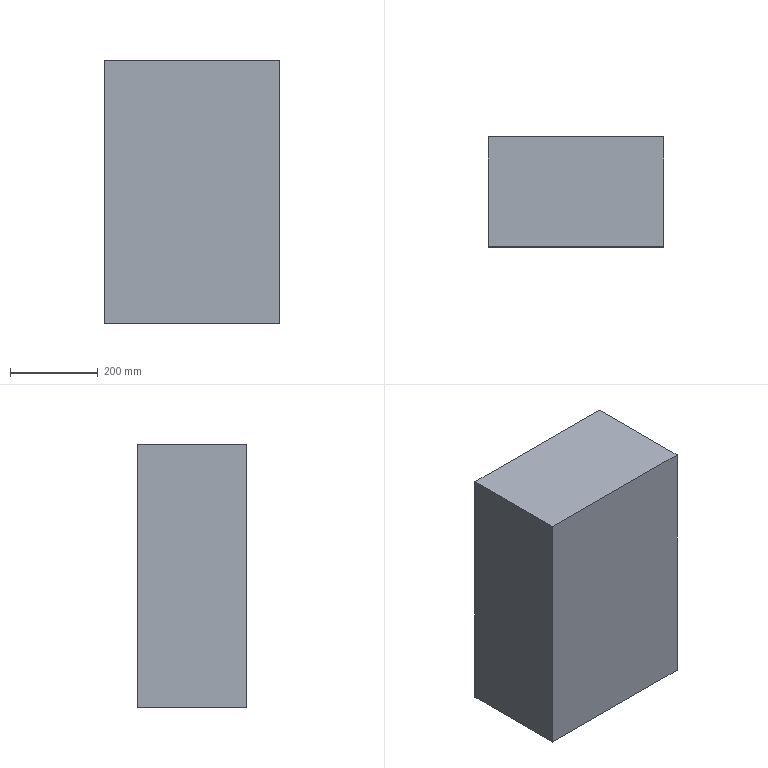Part | NX | features Hydrolic power unit 2 | 1 solid | 6 faces | box 400 x 250 x 600 mm | volume 60000000 mm3 | plane 6
STEP:
#1=CARTESIAN_POINT('',(-200.,-250.,-300.));
#2=VERTEX_POINT('',#1);
#3=CARTESIAN_POINT('',(-200.,-250.,300.));
#4=VERTEX_POINT('',#3);
#5=CARTESIAN_POINT('',(-200.,-250.,300.));
#6=DIRECTION('',(0.,0.,1.));
#7=VECTOR('',#6,1000.);
#8=LINE('',#5,#7);
#9=EDGE_CURVE('',#2,#4,#8,.T.);
#10=ORIENTED_EDGE('',*,*,#9,.T.);
#11=CARTESIAN_POINT('',(200.,-250.,300.));
#12=VERTEX_POINT('',#11);
#13=CARTESIAN_POINT('',(-200.,-250.,300.));
#14=DIRECTION('',(1.,0.,0.));
#15=VECTOR('',#14,1000.);
#16=LINE('',#13,#15);
#17=EDGE_CURVE('',#12,#4,#16,.F.);
#18=ORIENTED_EDGE('',*,*,#17,.F.);
#19=CARTESIAN_POINT('',(200.,-250.,-300.));
#20=VERTEX_POINT('',#19);
#21=CARTESIAN_POINT('',(200.,-250.,300.));
#22=DIRECTION('',(0.,0.,1.));
#23=VECTOR('',#22,1000.);
#24=LINE('',#21,#23);
#25=EDGE_CURVE('',#12,#20,#24,.F.);
#26=ORIENTED_EDGE('',*,*,#25,.T.);
#27=CARTESIAN_POINT('',(-200.,-250.,-300.));
#28=DIRECTION('',(1.,0.,0.));
#29=VECTOR('',#28,1000.);
#30=LINE('',#27,#29);
#31=EDGE_CURVE('',#20,#2,#30,.F.);
#32=ORIENTED_EDGE('',*,*,#31,.T.);
#33=EDGE_LOOP('',(#10,#18,#26,#32));
#34=FACE_BOUND('',#33,.T.);
#35=CARTESIAN_POINT('',(-200.,-250.,300.));
#36=DIRECTION('',(0.,-1.,0.));
#37=DIRECTION('',(0.,0.,-1.));
#38=AXIS2_PLACEMENT_3D('',#35,#36,#37);
#39=PLANE('',#38);
#40=ADVANCED_FACE('',(#34),#39,.F.);
#41=CARTESIAN_POINT('',(-200.,-500.,-300.));
#42=VERTEX_POINT('',#41);
#43=CARTESIAN_POINT('',(-200.,-500.,300.));
#44=VERTEX_POINT('',#43);
#45=CARTESIAN_POINT('',(-200.,-500.,300.));
#46=DIRECTION('',(0.,0.,1.));
#47=VECTOR('',#46,1000.);
#48=LINE('',#45,#47);
#49=EDGE_CURVE('',#42,#44,#48,.T.);
#50=ORIENTED_EDGE('',*,*,#49,.T.);
#51=CARTESIAN_POINT('',(-200.,-500.,300.));
#52=DIRECTION('',(0.,1.,0.));
#53=VECTOR('',#52,1000.);
#54=LINE('',#51,#53);
#55=EDGE_CURVE('',#4,#44,#54,.F.);
#56=ORIENTED_EDGE('',*,*,#55,.F.);
#57=ORIENTED_EDGE('',*,*,#9,.F.);
#58=CARTESIAN_POINT('',(-200.,-500.,-300.));
#59=DIRECTION('',(0.,1.,0.));
#60=VECTOR('',#59,1000.);
#61=LINE('',#58,#60);
#62=EDGE_CURVE('',#2,#42,#61,.F.);
#63=ORIENTED_EDGE('',*,*,#62,.T.);
#64=EDGE_LOOP('',(#50,#56,#57,#63));
#65=FACE_BOUND('',#64,.T.);
#66=CARTESIAN_POINT('',(-200.,-250.,300.));
#67=DIRECTION('',(1.,0.,0.));
#68=DIRECTION('',(0.,1.,0.));
#69=AXIS2_PLACEMENT_3D('',#66,#67,#68);
#70=PLANE('',#69);
#71=ADVANCED_FACE('',(#65),#70,.F.);
#72=CARTESIAN_POINT('',(200.,-500.,300.));
#73=VERTEX_POINT('',#72);
#74=CARTESIAN_POINT('',(200.,-250.,300.));
#75=DIRECTION('',(0.,-1.,0.));
#76=VECTOR('',#75,1000.);
#77=LINE('',#74,#76);
#78=EDGE_CURVE('',#73,#12,#77,.F.);
#79=ORIENTED_EDGE('',*,*,#78,.T.);
#80=ORIENTED_EDGE('',*,*,#17,.T.);
#81=ORIENTED_EDGE('',*,*,#55,.T.);
#82=CARTESIAN_POINT('',(-200.,-500.,300.));
#83=DIRECTION('',(1.,0.,0.));
#84=VECTOR('',#83,1000.);
#85=LINE('',#82,#84);
#86=EDGE_CURVE('',#44,#73,#85,.T.);
#87=ORIENTED_EDGE('',*,*,#86,.T.);
#88=EDGE_LOOP('',(#79,#80,#81,#87));
#89=FACE_BOUND('',#88,.T.);
#90=CARTESIAN_POINT('',(-200.,-500.,300.));
#91=DIRECTION('',(0.,0.,1.));
#92=DIRECTION('',(1.,0.,0.));
#93=AXIS2_PLACEMENT_3D('',#90,#91,#92);
#94=PLANE('',#93);
#95=ADVANCED_FACE('',(#89),#94,.T.);
#96=ORIENTED_EDGE('',*,*,#25,.F.);
#97=ORIENTED_EDGE('',*,*,#78,.F.);
#98=CARTESIAN_POINT('',(200.,-500.,-300.));
#99=VERTEX_POINT('',#98);
#100=CARTESIAN_POINT('',(200.,-500.,300.));
#101=DIRECTION('',(0.,0.,1.));
#102=VECTOR('',#101,1000.);
#103=LINE('',#100,#102);
#104=EDGE_CURVE('',#73,#99,#103,.F.);
#105=ORIENTED_EDGE('',*,*,#104,.T.);
#106=CARTESIAN_POINT('',(200.,-500.,-300.));
#107=DIRECTION('',(0.,1.,0.));
#108=VECTOR('',#107,1000.);
#109=LINE('',#106,#108);
#110=EDGE_CURVE('',#99,#20,#109,.T.);
#111=ORIENTED_EDGE('',*,*,#110,.T.);
#112=EDGE_LOOP('',(#96,#97,#105,#111));
#113=FACE_BOUND('',#112,.T.);
#114=CARTESIAN_POINT('',(200.,-250.,300.));
#115=DIRECTION('',(-1.,0.,0.));
#116=DIRECTION('',(0.,-1.,0.));
#117=AXIS2_PLACEMENT_3D('',#114,#115,#116);
#118=PLANE('',#117);
#119=ADVANCED_FACE('',(#113),#118,.F.);
#120=ORIENTED_EDGE('',*,*,#31,.F.);
#121=ORIENTED_EDGE('',*,*,#110,.F.);
#122=CARTESIAN_POINT('',(-200.,-500.,-300.));
#123=DIRECTION('',(1.,0.,0.));
#124=VECTOR('',#123,1000.);
#125=LINE('',#122,#124);
#126=EDGE_CURVE('',#99,#42,#125,.F.);
#127=ORIENTED_EDGE('',*,*,#126,.T.);
#128=ORIENTED_EDGE('',*,*,#62,.F.);
#129=EDGE_LOOP('',(#120,#121,#127,#128));
#130=FACE_BOUND('',#129,.T.);
#131=CARTESIAN_POINT('',(-200.,-500.,-300.));
#132=DIRECTION('',(0.,0.,1.));
#133=DIRECTION('',(1.,0.,0.));
#134=AXIS2_PLACEMENT_3D('',#131,#132,#133);
#135=PLANE('',#134);
#136=ADVANCED_FACE('',(#130),#135,.F.);
#137=ORIENTED_EDGE('',*,*,#104,.F.);
#138=ORIENTED_EDGE('',*,*,#86,.F.);
#139=ORIENTED_EDGE('',*,*,#49,.F.);
#140=ORIENTED_EDGE('',*,*,#126,.F.);
#141=EDGE_LOOP('',(#137,#138,#139,#140));
#142=FACE_BOUND('',#141,.T.);
#143=CARTESIAN_POINT('',(-200.,-500.,300.));
#144=DIRECTION('',(0.,1.,0.));
#145=DIRECTION('',(0.,0.,1.));
#146=AXIS2_PLACEMENT_3D('',#143,#144,#145);
#147=PLANE('',#146);
#148=ADVANCED_FACE('',(#142),#147,.F.);
#149=CLOSED_SHELL('',(#40,#71,#95,#119,#136,#148));
#150=MANIFOLD_SOLID_BREP('',#149);
#151=(LENGTH_UNIT()NAMED_UNIT(*)SI_UNIT(.MILLI.,.METRE.));
#152=UNCERTAINTY_MEASURE_WITH_UNIT(LENGTH_MEASURE(0.00001),#151,'','');
#153=(NAMED_UNIT(*)PLANE_ANGLE_UNIT()SI_UNIT($,.RADIAN.));
#154=(NAMED_UNIT(*)SI_UNIT($,.STERADIAN.)SOLID_ANGLE_UNIT());
#155=(GEOMETRIC_REPRESENTATION_CONTEXT(3)GLOBAL_UNCERTAINTY_ASSIGNED_CONTEXT((#152))GLOBAL_UNIT_ASSIGNED_CONTEXT((#151,#153,#154))REPRESENTATION_CONTEXT('',''));
#156=ADVANCED_BREP_SHAPE_REPRESENTATION('',(#150),#155);